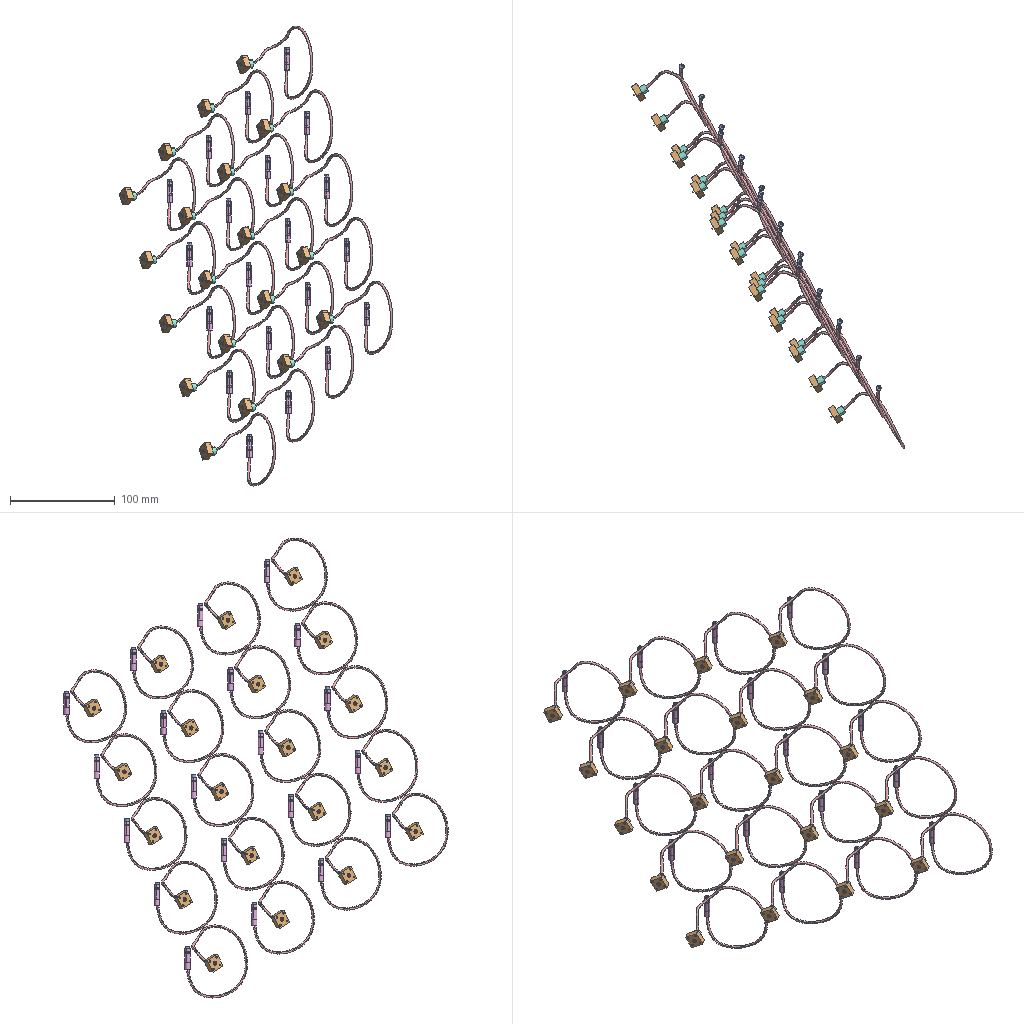Assembly | SolidWorks | 6 different items | 120 placed | box 261 x 367 x 439 mm
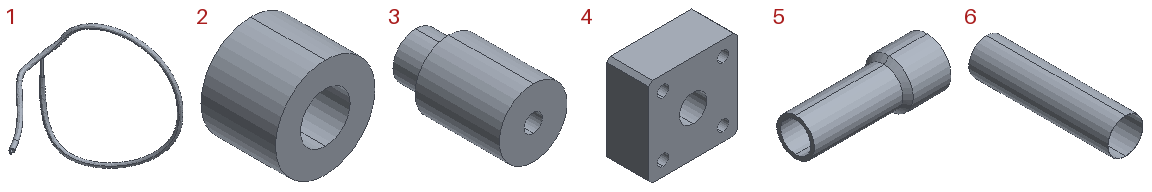Parts list (item | quantity | size | volume | features):
1 | x20 | 70.611 x 58.67 x 69.854 mm | 1093 mm3 | features 3DProfileFeature 2, ICE 2, Sweep 1
2 | x20 | 8 x 6 x 8 mm | 226.195 mm3 | features Revolution 1
3 | x20 | 4.1 x 7.1 x 4.1 mm | 72.551 mm3 | features Revolution 1
4 | x20 | 12.63 x 6 x 12.63 mm | 834.171 mm3 | features Extrusion 1, HoleWzd 1
5 | x20 | 13.74 x 5 x 5 mm | 67.776 mm3 | features Revolution 1
6 | x20 | 5.1 x 20 x 5.1 mm | 15.865 mm3 | features ExtruThin 1
Mates (type | each side: item.copy, entity, surface, feature):
Concentric | 1.1 edge | 3.1 edge
Concentric | 3.1 face cylinder Revolve1 | 5.1 face cylinder Revolve1
Concentric | 5.1 face cylinder Revolve1 | 6.1 face cylinder Extrude-Thin1
Coincident | 5.1 face plane Revolve1 | 6.1 face plane Extrude-Thin1
Concentric | 1.1 face cylinder Sweep1 | 2.1 face cylinder Revolve1
Concentric | 1.1 face cylinder Sweep1 | 4.1 face cylinder Boss-Extrude1
Coincident | 1.1 face plane Sweep1 | 4.1 face plane Boss-Extrude1
Coincident | 2.1 face plane Revolve1 | 4.1 face plane Boss-Extrude1